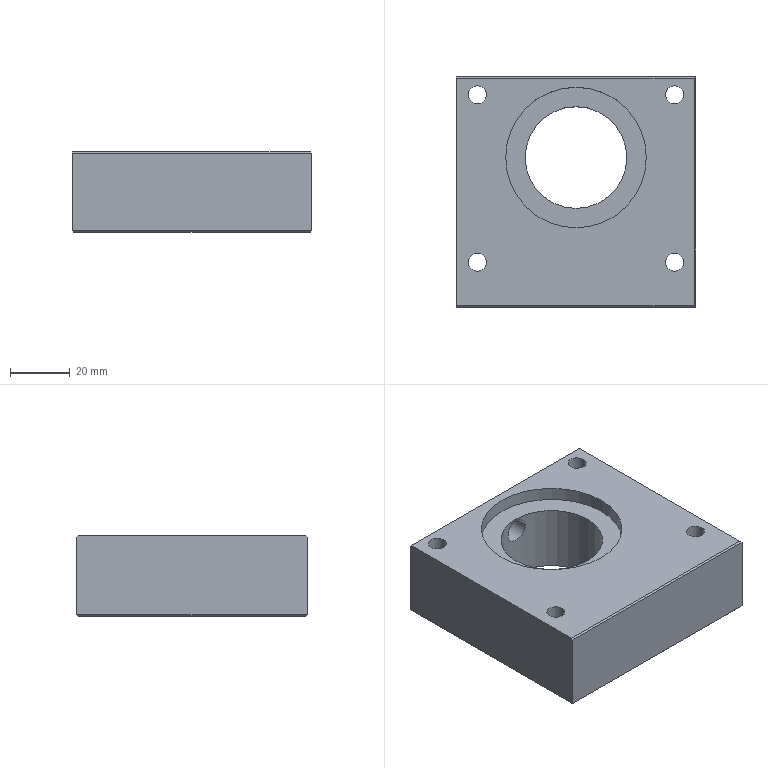Part | NX | 1 solid | 64 faces | box 80 x 77 x 27 mm | volume 132577 mm3 | cylinder 30 | plane 18 | cone 16 | commonest cylinder face diameters 4.2 x8 6 x8 9.5 x8 8 x2 34 x2 47 x2